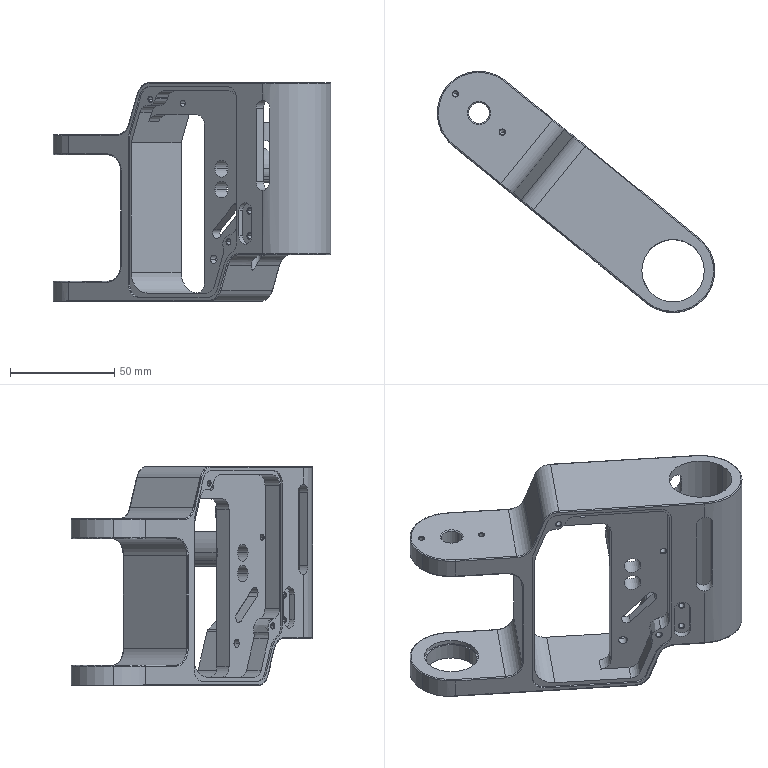Part | SolidWorks | features BaseBody 1 | 1 solid | 299 faces | box 133.101 x 115.712 x 105 mm | volume 145197 mm3 | cylinder 131 | plane 76 | cone 58 | spline 34 | commonest cylinder face diameters 10 x22 1 x20 2.5 x18 12 x13 8 x8 16 x7